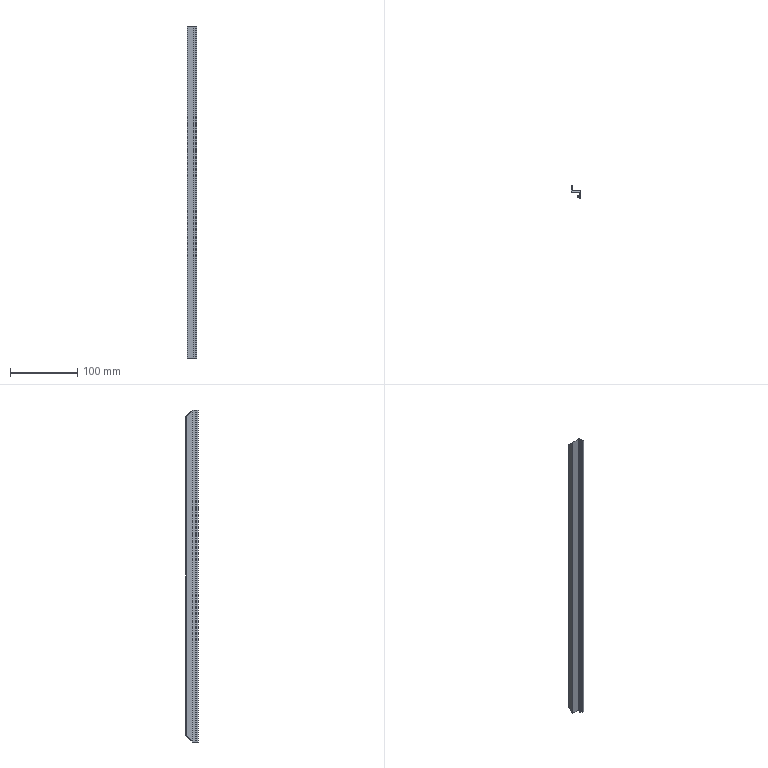Part | NX | features BREP 1 | 1 solid | 19 faces | box 14.9 x 19.1 x 494.9 mm | volume 34982 mm3 | plane 16 | cylinder 3 | commonest cylinder face diameters 1 x2 2 x1
STEP:
#1=CARTESIAN_POINT('',(12.9,-1.,245.95));
#2=VERTEX_POINT('',#1);
#3=CARTESIAN_POINT('',(12.9,-1.,-245.95));
#4=VERTEX_POINT('',#3);
#5=CARTESIAN_POINT('',(12.9,-1.,247.45));
#6=DIRECTION('',(0.,0.,-1.));
#7=VECTOR('',#6,1000.);
#8=LINE('',#5,#7);
#9=EDGE_CURVE('',#2,#4,#8,.T.);
#10=ORIENTED_EDGE('',*,*,#9,.T.);
#11=CARTESIAN_POINT('',(12.4,-0.5,-245.45));
#12=VERTEX_POINT('',#11);
#13=CARTESIAN_POINT('',(12.9,-1.,-245.95));
#14=CARTESIAN_POINT('',(12.9,-0.7071,-245.657));
#15=CARTESIAN_POINT('',(12.693,-0.5,-245.45));
#16=CARTESIAN_POINT('',(12.4,-0.5,-245.45));
#17=(BOUNDED_CURVE()B_SPLINE_CURVE(3,(#13,#14,#15,#16),.UNSPECIFIED.,.F.,.F.)B_SPLINE_CURVE_WITH_KNOTS((4,4),(1.571,3.142),.UNSPECIFIED.)CURVE()GEOMETRIC_REPRESENTATION_ITEM()RATIONAL_B_SPLINE_CURVE((1.,0.8047,0.8047,1.))REPRESENTATION_ITEM(''));
#18=EDGE_CURVE('',#4,#12,#17,.T.);
#19=ORIENTED_EDGE('',*,*,#18,.T.);
#20=CARTESIAN_POINT('',(12.4,-0.5,245.45));
#21=VERTEX_POINT('',#20);
#22=CARTESIAN_POINT('',(12.4,-0.5,247.45));
#23=DIRECTION('',(0.,0.,-1.));
#24=VECTOR('',#23,1000.);
#25=LINE('',#22,#24);
#26=EDGE_CURVE('',#21,#12,#25,.T.);
#27=ORIENTED_EDGE('',*,*,#26,.F.);
#28=CARTESIAN_POINT('',(12.4,-0.5,245.45));
#29=CARTESIAN_POINT('',(12.693,-0.5,245.45));
#30=CARTESIAN_POINT('',(12.9,-0.7071,245.657));
#31=CARTESIAN_POINT('',(12.9,-1.,245.95));
#32=(BOUNDED_CURVE()B_SPLINE_CURVE(3,(#28,#29,#30,#31),.UNSPECIFIED.,.F.,.F.)B_SPLINE_CURVE_WITH_KNOTS((4,4),(0.,1.571),.UNSPECIFIED.)CURVE()GEOMETRIC_REPRESENTATION_ITEM()RATIONAL_B_SPLINE_CURVE((1.,0.8047,0.8047,1.))REPRESENTATION_ITEM(''));
#33=EDGE_CURVE('',#21,#2,#32,.T.);
#34=ORIENTED_EDGE('',*,*,#33,.T.);
#35=EDGE_LOOP('',(#10,#19,#27,#34));
#36=FACE_BOUND('',#35,.T.);
#37=CARTESIAN_POINT('',(12.4,-1.,247.45));
#38=DIRECTION('',(0.,0.,-1.));
#39=DIRECTION('',(-1.,0.,0.));
#40=AXIS2_PLACEMENT_3D('',#37,#38,#39);
#41=CYLINDRICAL_SURFACE('',#40,0.5);
#42=ADVANCED_FACE('',(#36),#41,.T.);
#43=ORIENTED_EDGE('',*,*,#26,.T.);
#44=CARTESIAN_POINT('',(0.,-0.5,-245.45));
#45=VERTEX_POINT('',#44);
#46=CARTESIAN_POINT('',(0.,-0.5,-245.45));
#47=DIRECTION('',(-1.,0.,0.));
#48=VECTOR('',#47,1000.);
#49=LINE('',#46,#48);
#50=EDGE_CURVE('',#12,#45,#49,.T.);
#51=ORIENTED_EDGE('',*,*,#50,.T.);
#52=CARTESIAN_POINT('',(0.,-0.5,245.45));
#53=VERTEX_POINT('',#52);
#54=CARTESIAN_POINT('',(0.,-0.5,247.45));
#55=DIRECTION('',(0.,0.,-1.));
#56=VECTOR('',#55,1000.);
#57=LINE('',#54,#56);
#58=EDGE_CURVE('',#53,#45,#57,.T.);
#59=ORIENTED_EDGE('',*,*,#58,.F.);
#60=CARTESIAN_POINT('',(12.4,-0.5,245.45));
#61=DIRECTION('',(1.,0.,0.));
#62=VECTOR('',#61,1000.);
#63=LINE('',#60,#62);
#64=EDGE_CURVE('',#53,#21,#63,.T.);
#65=ORIENTED_EDGE('',*,*,#64,.T.);
#66=EDGE_LOOP('',(#43,#51,#59,#65));
#67=FACE_BOUND('',#66,.T.);
#68=CARTESIAN_POINT('',(12.4,-0.5,247.45));
#69=DIRECTION('',(0.,-1.,0.));
#70=DIRECTION('',(0.,0.,-1.));
#71=AXIS2_PLACEMENT_3D('',#68,#69,#70);
#72=PLANE('',#71);
#73=ADVANCED_FACE('',(#67),#72,.F.);
#74=ORIENTED_EDGE('',*,*,#58,.T.);
#75=CARTESIAN_POINT('',(0.,7.5,-237.45));
#76=VERTEX_POINT('',#75);
#77=CARTESIAN_POINT('',(0.,7.5,-237.45));
#78=DIRECTION('',(0.,0.7071,0.7071));
#79=VECTOR('',#78,1000.);
#80=LINE('',#77,#79);
#81=EDGE_CURVE('',#45,#76,#80,.T.);
#82=ORIENTED_EDGE('',*,*,#81,.T.);
#83=CARTESIAN_POINT('',(0.,7.5,237.45));
#84=VERTEX_POINT('',#83);
#85=CARTESIAN_POINT('',(0.,7.5,247.45));
#86=DIRECTION('',(0.,0.,-1.));
#87=VECTOR('',#86,1000.);
#88=LINE('',#85,#87);
#89=EDGE_CURVE('',#84,#76,#88,.T.);
#90=ORIENTED_EDGE('',*,*,#89,.F.);
#91=CARTESIAN_POINT('',(0.,-2.5,247.45));
#92=DIRECTION('',(0.,-0.7071,0.7071));
#93=VECTOR('',#92,1000.);
#94=LINE('',#91,#93);
#95=EDGE_CURVE('',#84,#53,#94,.T.);
#96=ORIENTED_EDGE('',*,*,#95,.T.);
#97=EDGE_LOOP('',(#74,#82,#90,#96));
#98=FACE_BOUND('',#97,.T.);
#99=CARTESIAN_POINT('',(0.,-0.5,247.45));
#100=DIRECTION('',(-1.,0.,0.));
#101=DIRECTION('',(0.,0.,1.));
#102=AXIS2_PLACEMENT_3D('',#99,#100,#101);
#103=PLANE('',#102);
#104=ADVANCED_FACE('',(#98),#103,.F.);
#105=ORIENTED_EDGE('',*,*,#89,.T.);
#106=CARTESIAN_POINT('',(-1.,7.5,-237.45));
#107=VERTEX_POINT('',#106);
#108=CARTESIAN_POINT('',(0.,7.5,-237.45));
#109=DIRECTION('',(-1.,0.,0.));
#110=VECTOR('',#109,1000.);
#111=LINE('',#108,#110);
#112=EDGE_CURVE('',#76,#107,#111,.T.);
#113=ORIENTED_EDGE('',*,*,#112,.T.);
#114=CARTESIAN_POINT('',(-1.,7.5,237.45));
#115=VERTEX_POINT('',#114);
#116=CARTESIAN_POINT('',(-1.,7.5,247.45));
#117=DIRECTION('',(0.,0.,-1.));
#118=VECTOR('',#117,1000.);
#119=LINE('',#116,#118);
#120=EDGE_CURVE('',#115,#107,#119,.T.);
#121=ORIENTED_EDGE('',*,*,#120,.F.);
#122=CARTESIAN_POINT('',(0.,7.5,237.45));
#123=DIRECTION('',(1.,0.,0.));
#124=VECTOR('',#123,1000.);
#125=LINE('',#122,#124);
#126=EDGE_CURVE('',#115,#84,#125,.T.);
#127=ORIENTED_EDGE('',*,*,#126,.T.);
#128=EDGE_LOOP('',(#105,#113,#121,#127));
#129=FACE_BOUND('',#128,.T.);
#130=CARTESIAN_POINT('',(0.,7.5,247.45));
#131=DIRECTION('',(0.,-1.,0.));
#132=DIRECTION('',(0.,0.,-1.));
#133=AXIS2_PLACEMENT_3D('',#130,#131,#132);
#134=PLANE('',#133);
#135=ADVANCED_FACE('',(#129),#134,.F.);
#136=ORIENTED_EDGE('',*,*,#120,.T.);
#137=CARTESIAN_POINT('',(-2.,6.5,-238.45));
#138=VERTEX_POINT('',#137);
#139=CARTESIAN_POINT('',(-1.,7.5,-237.45));
#140=CARTESIAN_POINT('',(-1.586,7.5,-237.45));
#141=CARTESIAN_POINT('',(-2.,7.086,-237.864));
#142=CARTESIAN_POINT('',(-2.,6.5,-238.45));
#143=(BOUNDED_CURVE()B_SPLINE_CURVE(3,(#139,#140,#141,#142),.UNSPECIFIED.,.F.,.F.)B_SPLINE_CURVE_WITH_KNOTS((4,4),(3.142,4.712),.UNSPECIFIED.)CURVE()GEOMETRIC_REPRESENTATION_ITEM()RATIONAL_B_SPLINE_CURVE((1.,0.8047,0.8047,1.))REPRESENTATION_ITEM(''));
#144=EDGE_CURVE('',#107,#138,#143,.T.);
#145=ORIENTED_EDGE('',*,*,#144,.T.);
#146=CARTESIAN_POINT('',(-2.,6.5,238.45));
#147=VERTEX_POINT('',#146);
#148=CARTESIAN_POINT('',(-2.,6.5,247.45));
#149=DIRECTION('',(0.,0.,-1.));
#150=VECTOR('',#149,1000.);
#151=LINE('',#148,#150);
#152=EDGE_CURVE('',#147,#138,#151,.T.);
#153=ORIENTED_EDGE('',*,*,#152,.F.);
#154=CARTESIAN_POINT('',(-2.,6.5,238.45));
#155=CARTESIAN_POINT('',(-2.,7.086,237.864));
#156=CARTESIAN_POINT('',(-1.586,7.5,237.45));
#157=CARTESIAN_POINT('',(-1.,7.5,237.45));
#158=(BOUNDED_CURVE()B_SPLINE_CURVE(3,(#154,#155,#156,#157),.UNSPECIFIED.,.F.,.F.)B_SPLINE_CURVE_WITH_KNOTS((4,4),(4.712,6.283),.UNSPECIFIED.)CURVE()GEOMETRIC_REPRESENTATION_ITEM()RATIONAL_B_SPLINE_CURVE((1.,0.8047,0.8047,1.))REPRESENTATION_ITEM(''));
#159=EDGE_CURVE('',#147,#115,#158,.T.);
#160=ORIENTED_EDGE('',*,*,#159,.T.);
#161=EDGE_LOOP('',(#136,#145,#153,#160));
#162=FACE_BOUND('',#161,.T.);
#163=CARTESIAN_POINT('',(-1.,6.5,247.45));
#164=DIRECTION('',(0.,0.,-1.));
#165=DIRECTION('',(-1.,0.,0.));
#166=AXIS2_PLACEMENT_3D('',#163,#164,#165);
#167=CYLINDRICAL_SURFACE('',#166,1.);
#168=ADVANCED_FACE('',(#162),#167,.T.);
#169=ORIENTED_EDGE('',*,*,#152,.T.);
#170=CARTESIAN_POINT('',(-2.,-2.5,-247.45));
#171=VERTEX_POINT('',#170);
#172=CARTESIAN_POINT('',(-2.,7.5,-237.45));
#173=DIRECTION('',(0.,-0.7071,-0.7071));
#174=VECTOR('',#173,1000.);
#175=LINE('',#172,#174);
#176=EDGE_CURVE('',#138,#171,#175,.T.);
#177=ORIENTED_EDGE('',*,*,#176,.T.);
#178=CARTESIAN_POINT('',(-2.,-2.5,247.45));
#179=VERTEX_POINT('',#178);
#180=CARTESIAN_POINT('',(-2.,-2.5,247.45));
#181=DIRECTION('',(0.,0.,-1.));
#182=VECTOR('',#181,1000.);
#183=LINE('',#180,#182);
#184=EDGE_CURVE('',#179,#171,#183,.T.);
#185=ORIENTED_EDGE('',*,*,#184,.F.);
#186=CARTESIAN_POINT('',(-2.,-2.5,247.45));
#187=DIRECTION('',(0.,0.7071,-0.7071));
#188=VECTOR('',#187,1000.);
#189=LINE('',#186,#188);
#190=EDGE_CURVE('',#179,#147,#189,.T.);
#191=ORIENTED_EDGE('',*,*,#190,.T.);
#192=EDGE_LOOP('',(#169,#177,#185,#191));
#193=FACE_BOUND('',#192,.T.);
#194=CARTESIAN_POINT('',(-2.,6.5,247.45));
#195=DIRECTION('',(1.,0.,0.));
#196=DIRECTION('',(0.,1.,0.));
#197=AXIS2_PLACEMENT_3D('',#194,#195,#196);
#198=PLANE('',#197);
#199=ADVANCED_FACE('',(#193),#198,.F.);
#200=CARTESIAN_POINT('',(10.4,-2.5,-247.45));
#201=VERTEX_POINT('',#200);
#202=CARTESIAN_POINT('',(-2.,-2.5,-247.45));
#203=DIRECTION('',(1.,0.,0.));
#204=VECTOR('',#203,1000.);
#205=LINE('',#202,#204);
#206=EDGE_CURVE('',#171,#201,#205,.T.);
#207=ORIENTED_EDGE('',*,*,#206,.T.);
#208=CARTESIAN_POINT('',(10.4,-2.5,247.45));
#209=VERTEX_POINT('',#208);
#210=CARTESIAN_POINT('',(10.4,-2.5,247.45));
#211=DIRECTION('',(0.,0.,-1.));
#212=VECTOR('',#211,1000.);
#213=LINE('',#210,#212);
#214=EDGE_CURVE('',#209,#201,#213,.T.);
#215=ORIENTED_EDGE('',*,*,#214,.F.);
#216=CARTESIAN_POINT('',(-2.,-2.5,247.45));
#217=DIRECTION('',(1.,0.,0.));
#218=VECTOR('',#217,1000.);
#219=LINE('',#216,#218);
#220=EDGE_CURVE('',#179,#209,#219,.T.);
#221=ORIENTED_EDGE('',*,*,#220,.F.);
#222=ORIENTED_EDGE('',*,*,#184,.T.);
#223=EDGE_LOOP('',(#207,#215,#221,#222));
#224=FACE_BOUND('',#223,.T.);
#225=CARTESIAN_POINT('',(-2.,-2.5,247.45));
#226=DIRECTION('',(0.,1.,0.));
#227=DIRECTION('',(1.,0.,0.));
#228=AXIS2_PLACEMENT_3D('',#225,#226,#227);
#229=PLANE('',#228);
#230=ADVANCED_FACE('',(#224),#229,.F.);
#231=CARTESIAN_POINT('',(10.9,-3.,-247.45));
#232=VERTEX_POINT('',#231);
#233=CARTESIAN_POINT('',(10.4,-3.,-247.45));
#234=DIRECTION('',(0.,0.,-1.));
#235=DIRECTION('',(1.,0.,0.));
#236=AXIS2_PLACEMENT_3D('',#233,#234,#235);
#237=CIRCLE('',#236,0.5);
#238=EDGE_CURVE('',#201,#232,#237,.T.);
#239=ORIENTED_EDGE('',*,*,#238,.T.);
#240=CARTESIAN_POINT('',(10.9,-3.,247.45));
#241=VERTEX_POINT('',#240);
#242=CARTESIAN_POINT('',(10.9,-3.,247.45));
#243=DIRECTION('',(0.,0.,-1.));
#244=VECTOR('',#243,1000.);
#245=LINE('',#242,#244);
#246=EDGE_CURVE('',#241,#232,#245,.T.);
#247=ORIENTED_EDGE('',*,*,#246,.F.);
#248=CARTESIAN_POINT('',(10.4,-3.,247.45));
#249=DIRECTION('',(0.,0.,-1.));
#250=DIRECTION('',(1.,0.,0.));
#251=AXIS2_PLACEMENT_3D('',#248,#249,#250);
#252=CIRCLE('',#251,0.5);
#253=EDGE_CURVE('',#209,#241,#252,.T.);
#254=ORIENTED_EDGE('',*,*,#253,.F.);
#255=ORIENTED_EDGE('',*,*,#214,.T.);
#256=EDGE_LOOP('',(#239,#247,#254,#255));
#257=FACE_BOUND('',#256,.T.);
#258=CARTESIAN_POINT('',(10.4,-3.,247.45));
#259=DIRECTION('',(0.,0.,-1.));
#260=DIRECTION('',(-1.,0.,0.));
#261=AXIS2_PLACEMENT_3D('',#258,#259,#260);
#262=CYLINDRICAL_SURFACE('',#261,0.5);
#263=ADVANCED_FACE('',(#257),#262,.F.);
#264=CARTESIAN_POINT('',(10.9,-7.2,-247.45));
#265=VERTEX_POINT('',#264);
#266=CARTESIAN_POINT('',(10.9,-3.,-247.45));
#267=DIRECTION('',(0.,-1.,0.));
#268=VECTOR('',#267,1000.);
#269=LINE('',#266,#268);
#270=EDGE_CURVE('',#232,#265,#269,.T.);
#271=ORIENTED_EDGE('',*,*,#270,.T.);
#272=CARTESIAN_POINT('',(10.9,-7.2,247.45));
#273=VERTEX_POINT('',#272);
#274=CARTESIAN_POINT('',(10.9,-7.2,247.45));
#275=DIRECTION('',(0.,0.,-1.));
#276=VECTOR('',#275,1000.);
#277=LINE('',#274,#276);
#278=EDGE_CURVE('',#273,#265,#277,.T.);
#279=ORIENTED_EDGE('',*,*,#278,.F.);
#280=CARTESIAN_POINT('',(10.9,-3.,247.45));
#281=DIRECTION('',(0.,-1.,0.));
#282=VECTOR('',#281,1000.);
#283=LINE('',#280,#282);
#284=EDGE_CURVE('',#241,#273,#283,.T.);
#285=ORIENTED_EDGE('',*,*,#284,.F.);
#286=ORIENTED_EDGE('',*,*,#246,.T.);
#287=EDGE_LOOP('',(#271,#279,#285,#286));
#288=FACE_BOUND('',#287,.T.);
#289=CARTESIAN_POINT('',(10.9,-3.,247.45));
#290=DIRECTION('',(1.,0.,0.));
#291=DIRECTION('',(0.,1.,0.));
#292=AXIS2_PLACEMENT_3D('',#289,#290,#291);
#293=PLANE('',#292);
#294=ADVANCED_FACE('',(#288),#293,.F.);
#295=CARTESIAN_POINT('',(7.2,-7.2,-247.45));
#296=VERTEX_POINT('',#295);
#297=CARTESIAN_POINT('',(10.9,-7.2,-247.45));
#298=DIRECTION('',(-1.,0.,0.));
#299=VECTOR('',#298,1000.);
#300=LINE('',#297,#299);
#301=EDGE_CURVE('',#265,#296,#300,.T.);
#302=ORIENTED_EDGE('',*,*,#301,.T.);
#303=CARTESIAN_POINT('',(7.2,-7.2,247.45));
#304=VERTEX_POINT('',#303);
#305=CARTESIAN_POINT('',(7.2,-7.2,247.45));
#306=DIRECTION('',(0.,0.,-1.));
#307=VECTOR('',#306,1000.);
#308=LINE('',#305,#307);
#309=EDGE_CURVE('',#304,#296,#308,.T.);
#310=ORIENTED_EDGE('',*,*,#309,.F.);
#311=CARTESIAN_POINT('',(10.9,-7.2,247.45));
#312=DIRECTION('',(-1.,0.,0.));
#313=VECTOR('',#312,1000.);
#314=LINE('',#311,#313);
#315=EDGE_CURVE('',#273,#304,#314,.T.);
#316=ORIENTED_EDGE('',*,*,#315,.F.);
#317=ORIENTED_EDGE('',*,*,#278,.T.);
#318=EDGE_LOOP('',(#302,#310,#316,#317));
#319=FACE_BOUND('',#318,.T.);
#320=CARTESIAN_POINT('',(10.9,-7.2,247.45));
#321=DIRECTION('',(0.,-1.,0.));
#322=DIRECTION('',(0.,0.,-1.));
#323=AXIS2_PLACEMENT_3D('',#320,#321,#322);
#324=PLANE('',#323);
#325=ADVANCED_FACE('',(#319),#324,.F.);
#326=CARTESIAN_POINT('',(7.2,-9.2,-247.45));
#327=VERTEX_POINT('',#326);
#328=CARTESIAN_POINT('',(7.2,-7.2,-247.45));
#329=DIRECTION('',(0.,-1.,0.));
#330=VECTOR('',#329,1000.);
#331=LINE('',#328,#330);
#332=EDGE_CURVE('',#296,#327,#331,.T.);
#333=ORIENTED_EDGE('',*,*,#332,.T.);
#334=CARTESIAN_POINT('',(7.2,-9.2,247.45));
#335=VERTEX_POINT('',#334);
#336=CARTESIAN_POINT('',(7.2,-9.2,247.45));
#337=DIRECTION('',(0.,0.,-1.));
#338=VECTOR('',#337,1000.);
#339=LINE('',#336,#338);
#340=EDGE_CURVE('',#335,#327,#339,.T.);
#341=ORIENTED_EDGE('',*,*,#340,.F.);
#342=CARTESIAN_POINT('',(7.2,-7.2,247.45));
#343=DIRECTION('',(0.,-1.,0.));
#344=VECTOR('',#343,1000.);
#345=LINE('',#342,#344);
#346=EDGE_CURVE('',#304,#335,#345,.T.);
#347=ORIENTED_EDGE('',*,*,#346,.F.);
#348=ORIENTED_EDGE('',*,*,#309,.T.);
#349=EDGE_LOOP('',(#333,#341,#347,#348));
#350=FACE_BOUND('',#349,.T.);
#351=CARTESIAN_POINT('',(7.2,-7.2,247.45));
#352=DIRECTION('',(1.,0.,0.));
#353=DIRECTION('',(0.,1.,0.));
#354=AXIS2_PLACEMENT_3D('',#351,#352,#353);
#355=PLANE('',#354);
#356=ADVANCED_FACE('',(#350),#355,.F.);
#357=CARTESIAN_POINT('',(10.9,-9.2,-247.45));
#358=VERTEX_POINT('',#357);
#359=CARTESIAN_POINT('',(7.2,-9.2,-247.45));
#360=DIRECTION('',(1.,0.,0.));
#361=VECTOR('',#360,1000.);
#362=LINE('',#359,#361);
#363=EDGE_CURVE('',#327,#358,#362,.T.);
#364=ORIENTED_EDGE('',*,*,#363,.T.);
#365=CARTESIAN_POINT('',(10.9,-9.2,247.45));
#366=VERTEX_POINT('',#365);
#367=CARTESIAN_POINT('',(10.9,-9.2,247.45));
#368=DIRECTION('',(0.,0.,-1.));
#369=VECTOR('',#368,1000.);
#370=LINE('',#367,#369);
#371=EDGE_CURVE('',#366,#358,#370,.T.);
#372=ORIENTED_EDGE('',*,*,#371,.F.);
#373=CARTESIAN_POINT('',(7.2,-9.2,247.45));
#374=DIRECTION('',(1.,0.,0.));
#375=VECTOR('',#374,1000.);
#376=LINE('',#373,#375);
#377=EDGE_CURVE('',#335,#366,#376,.T.);
#378=ORIENTED_EDGE('',*,*,#377,.F.);
#379=ORIENTED_EDGE('',*,*,#340,.T.);
#380=EDGE_LOOP('',(#364,#372,#378,#379));
#381=FACE_BOUND('',#380,.T.);
#382=CARTESIAN_POINT('',(7.2,-9.2,247.45));
#383=DIRECTION('',(0.,1.,0.));
#384=DIRECTION('',(1.,0.,0.));
#385=AXIS2_PLACEMENT_3D('',#382,#383,#384);
#386=PLANE('',#385);
#387=ADVANCED_FACE('',(#381),#386,.F.);
#388=CARTESIAN_POINT('',(10.9,-11.6,-247.45));
#389=VERTEX_POINT('',#388);
#390=CARTESIAN_POINT('',(10.9,-9.2,-247.45));
#391=DIRECTION('',(0.,-1.,0.));
#392=VECTOR('',#391,1000.);
#393=LINE('',#390,#392);
#394=EDGE_CURVE('',#358,#389,#393,.T.);
#395=ORIENTED_EDGE('',*,*,#394,.T.);
#396=CARTESIAN_POINT('',(10.9,-11.6,247.45));
#397=VERTEX_POINT('',#396);
#398=CARTESIAN_POINT('',(10.9,-11.6,247.45));
#399=DIRECTION('',(0.,0.,-1.));
#400=VECTOR('',#399,1000.);
#401=LINE('',#398,#400);
#402=EDGE_CURVE('',#397,#389,#401,.T.);
#403=ORIENTED_EDGE('',*,*,#402,.F.);
#404=CARTESIAN_POINT('',(10.9,-9.2,247.45));
#405=DIRECTION('',(0.,-1.,0.));
#406=VECTOR('',#405,1000.);
#407=LINE('',#404,#406);
#408=EDGE_CURVE('',#366,#397,#407,.T.);
#409=ORIENTED_EDGE('',*,*,#408,.F.);
#410=ORIENTED_EDGE('',*,*,#371,.T.);
#411=EDGE_LOOP('',(#395,#403,#409,#410));
#412=FACE_BOUND('',#411,.T.);
#413=CARTESIAN_POINT('',(10.9,-9.2,247.45));
#414=DIRECTION('',(1.,0.,0.));
#415=DIRECTION('',(0.,1.,0.));
#416=AXIS2_PLACEMENT_3D('',#413,#414,#415);
#417=PLANE('',#416);
#418=ADVANCED_FACE('',(#412),#417,.F.);
#419=CARTESIAN_POINT('',(12.9,-11.6,-247.45));
#420=VERTEX_POINT('',#419);
#421=CARTESIAN_POINT('',(10.9,-11.6,-247.45));
#422=DIRECTION('',(1.,0.,0.));
#423=VECTOR('',#422,1000.);
#424=LINE('',#421,#423);
#425=EDGE_CURVE('',#389,#420,#424,.T.);
#426=ORIENTED_EDGE('',*,*,#425,.T.);
#427=CARTESIAN_POINT('',(12.9,-11.6,247.45));
#428=VERTEX_POINT('',#427);
#429=CARTESIAN_POINT('',(12.9,-11.6,247.45));
#430=DIRECTION('',(0.,0.,-1.));
#431=VECTOR('',#430,1000.);
#432=LINE('',#429,#431);
#433=EDGE_CURVE('',#428,#420,#432,.T.);
#434=ORIENTED_EDGE('',*,*,#433,.F.);
#435=CARTESIAN_POINT('',(10.9,-11.6,247.45));
#436=DIRECTION('',(1.,0.,0.));
#437=VECTOR('',#436,1000.);
#438=LINE('',#435,#437);
#439=EDGE_CURVE('',#397,#428,#438,.T.);
#440=ORIENTED_EDGE('',*,*,#439,.F.);
#441=ORIENTED_EDGE('',*,*,#402,.T.);
#442=EDGE_LOOP('',(#426,#434,#440,#441));
#443=FACE_BOUND('',#442,.T.);
#444=CARTESIAN_POINT('',(10.9,-11.6,247.45));
#445=DIRECTION('',(0.,1.,0.));
#446=DIRECTION('',(1.,0.,0.));
#447=AXIS2_PLACEMENT_3D('',#444,#445,#446);
#448=PLANE('',#447);
#449=ADVANCED_FACE('',(#443),#448,.F.);
#450=CARTESIAN_POINT('',(12.9,-2.5,-247.45));
#451=VERTEX_POINT('',#450);
#452=CARTESIAN_POINT('',(12.9,-11.6,-247.45));
#453=DIRECTION('',(0.,1.,0.));
#454=VECTOR('',#453,1000.);
#455=LINE('',#452,#454);
#456=EDGE_CURVE('',#420,#451,#455,.T.);
#457=ORIENTED_EDGE('',*,*,#456,.T.);
#458=CARTESIAN_POINT('',(12.9,7.5,-237.45));
#459=DIRECTION('',(0.,0.7071,0.7071));
#460=VECTOR('',#459,1000.);
#461=LINE('',#458,#460);
#462=EDGE_CURVE('',#451,#4,#461,.T.);
#463=ORIENTED_EDGE('',*,*,#462,.T.);
#464=ORIENTED_EDGE('',*,*,#9,.F.);
#465=CARTESIAN_POINT('',(12.9,-2.5,247.45));
#466=VERTEX_POINT('',#465);
#467=CARTESIAN_POINT('',(12.9,-2.5,247.45));
#468=DIRECTION('',(0.,-0.7071,0.7071));
#469=VECTOR('',#468,1000.);
#470=LINE('',#467,#469);
#471=EDGE_CURVE('',#2,#466,#470,.T.);
#472=ORIENTED_EDGE('',*,*,#471,.T.);
#473=CARTESIAN_POINT('',(12.9,-11.6,247.45));
#474=DIRECTION('',(0.,1.,0.));
#475=VECTOR('',#474,1000.);
#476=LINE('',#473,#475);
#477=EDGE_CURVE('',#428,#466,#476,.T.);
#478=ORIENTED_EDGE('',*,*,#477,.F.);
#479=ORIENTED_EDGE('',*,*,#433,.T.);
#480=EDGE_LOOP('',(#457,#463,#464,#472,#478,#479));
#481=FACE_BOUND('',#480,.T.);
#482=CARTESIAN_POINT('',(12.9,-11.6,247.45));
#483=DIRECTION('',(-1.,0.,0.));
#484=DIRECTION('',(0.,1.,0.));
#485=AXIS2_PLACEMENT_3D('',#482,#483,#484);
#486=PLANE('',#485);
#487=ADVANCED_FACE('',(#481),#486,.F.);
#488=ORIENTED_EDGE('',*,*,#477,.T.);
#489=CARTESIAN_POINT('',(-1.,-2.5,247.45));
#490=DIRECTION('',(-1.,0.,0.));
#491=VECTOR('',#490,1000.);
#492=LINE('',#489,#491);
#493=EDGE_CURVE('',#466,#209,#492,.T.);
#494=ORIENTED_EDGE('',*,*,#493,.T.);
#495=ORIENTED_EDGE('',*,*,#253,.T.);
#496=ORIENTED_EDGE('',*,*,#284,.T.);
#497=ORIENTED_EDGE('',*,*,#315,.T.);
#498=ORIENTED_EDGE('',*,*,#346,.T.);
#499=ORIENTED_EDGE('',*,*,#377,.T.);
#500=ORIENTED_EDGE('',*,*,#408,.T.);
#501=ORIENTED_EDGE('',*,*,#439,.T.);
#502=EDGE_LOOP('',(#488,#494,#495,#496,#497,#498,#499,#500,#501));
#503=FACE_BOUND('',#502,.T.);
#504=CARTESIAN_POINT('',(12.4,-1.,247.45));
#505=DIRECTION('',(0.,0.,1.));
#506=DIRECTION('',(1.,0.,0.));
#507=AXIS2_PLACEMENT_3D('',#504,#505,#506);
#508=PLANE('',#507);
#509=ADVANCED_FACE('',(#503),#508,.T.);
#510=ORIENTED_EDGE('',*,*,#238,.F.);
#511=CARTESIAN_POINT('',(12.4,-2.5,-247.45));
#512=DIRECTION('',(1.,0.,0.));
#513=VECTOR('',#512,1000.);
#514=LINE('',#511,#513);
#515=EDGE_CURVE('',#201,#451,#514,.T.);
#516=ORIENTED_EDGE('',*,*,#515,.T.);
#517=ORIENTED_EDGE('',*,*,#456,.F.);
#518=ORIENTED_EDGE('',*,*,#425,.F.);
#519=ORIENTED_EDGE('',*,*,#394,.F.);
#520=ORIENTED_EDGE('',*,*,#363,.F.);
#521=ORIENTED_EDGE('',*,*,#332,.F.);
#522=ORIENTED_EDGE('',*,*,#301,.F.);
#523=ORIENTED_EDGE('',*,*,#270,.F.);
#524=EDGE_LOOP('',(#510,#516,#517,#518,#519,#520,#521,#522,#523));
#525=FACE_BOUND('',#524,.T.);
#526=CARTESIAN_POINT('',(12.4,-1.,-247.45));
#527=DIRECTION('',(0.,0.,1.));
#528=DIRECTION('',(1.,0.,0.));
#529=AXIS2_PLACEMENT_3D('',#526,#527,#528);
#530=PLANE('',#529);
#531=ADVANCED_FACE('',(#525),#530,.F.);
#532=ORIENTED_EDGE('',*,*,#515,.F.);
#533=ORIENTED_EDGE('',*,*,#206,.F.);
#534=ORIENTED_EDGE('',*,*,#176,.F.);
#535=ORIENTED_EDGE('',*,*,#144,.F.);
#536=ORIENTED_EDGE('',*,*,#112,.F.);
#537=ORIENTED_EDGE('',*,*,#81,.F.);
#538=ORIENTED_EDGE('',*,*,#50,.F.);
#539=ORIENTED_EDGE('',*,*,#18,.F.);
#540=ORIENTED_EDGE('',*,*,#462,.F.);
#541=EDGE_LOOP('',(#532,#533,#534,#535,#536,#537,#538,#539,#540));
#542=FACE_BOUND('',#541,.T.);
#543=CARTESIAN_POINT('',(0.,7.5,-237.45));
#544=DIRECTION('',(0.,-0.7071,0.7071));
#545=DIRECTION('',(-1.,0.,0.));
#546=AXIS2_PLACEMENT_3D('',#543,#544,#545);
#547=PLANE('',#546);
#548=ADVANCED_FACE('',(#542),#547,.F.);
#549=ORIENTED_EDGE('',*,*,#95,.F.);
#550=ORIENTED_EDGE('',*,*,#126,.F.);
#551=ORIENTED_EDGE('',*,*,#159,.F.);
#552=ORIENTED_EDGE('',*,*,#190,.F.);
#553=ORIENTED_EDGE('',*,*,#220,.T.);
#554=ORIENTED_EDGE('',*,*,#493,.F.);
#555=ORIENTED_EDGE('',*,*,#471,.F.);
#556=ORIENTED_EDGE('',*,*,#33,.F.);
#557=ORIENTED_EDGE('',*,*,#64,.F.);
#558=EDGE_LOOP('',(#549,#550,#551,#552,#553,#554,#555,#556,#557));
#559=FACE_BOUND('',#558,.T.);
#560=CARTESIAN_POINT('',(12.4,-2.5,247.45));
#561=DIRECTION('',(0.,0.7071,0.7071));
#562=DIRECTION('',(1.,0.,0.));
#563=AXIS2_PLACEMENT_3D('',#560,#561,#562);
#564=PLANE('',#563);
#565=ADVANCED_FACE('',(#559),#564,.T.);
#566=CLOSED_SHELL('',(#42,#73,#104,#135,#168,#199,#230,#263,#294,#325,#356,#387,#418,#449,#487,#509,#531,#548,#565));
#567=MANIFOLD_SOLID_BREP('',#566);
#568=(LENGTH_UNIT()NAMED_UNIT(*)SI_UNIT(.MILLI.,.METRE.));
#569=UNCERTAINTY_MEASURE_WITH_UNIT(LENGTH_MEASURE(0.00001),#568,'','');
#570=(NAMED_UNIT(*)PLANE_ANGLE_UNIT()SI_UNIT($,.RADIAN.));
#571=(NAMED_UNIT(*)SI_UNIT($,.STERADIAN.)SOLID_ANGLE_UNIT());
#572=(GEOMETRIC_REPRESENTATION_CONTEXT(3)GLOBAL_UNCERTAINTY_ASSIGNED_CONTEXT((#569))GLOBAL_UNIT_ASSIGNED_CONTEXT((#568,#570,#571))REPRESENTATION_CONTEXT('',''));
#573=ADVANCED_BREP_SHAPE_REPRESENTATION('',(#567),#572);